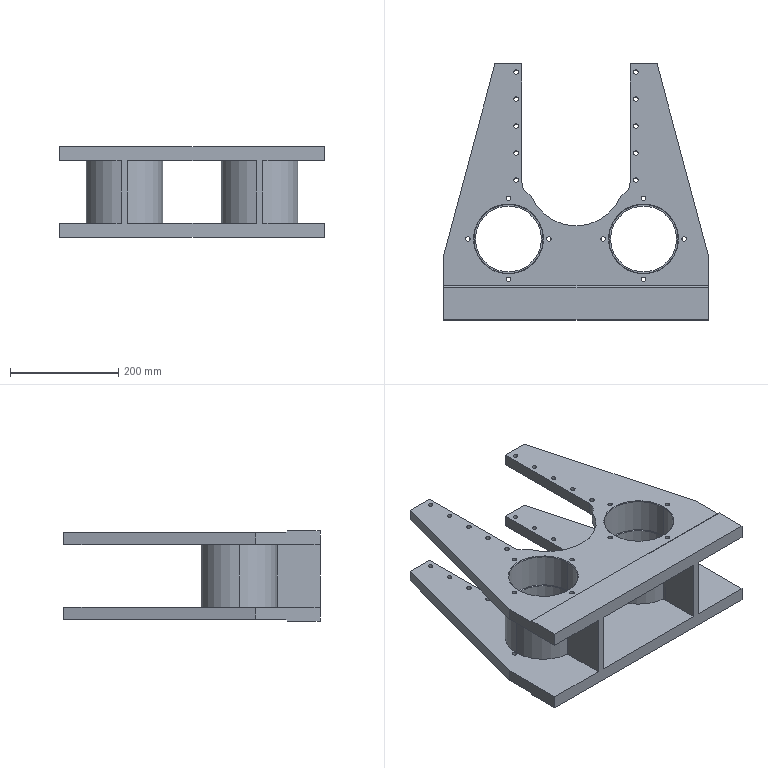Part | SolidWorks | features BaseBody 1 | 1 solid | 149 faces | box 490 x 474 x 167.3 mm | volume 6268436 mm3 | cylinder 100 | plane 33 | cone 16 | commonest cylinder face diameters 8.376 x68 10.106 x8 128 x8 141.3 x6 50 x4 122.24 x4